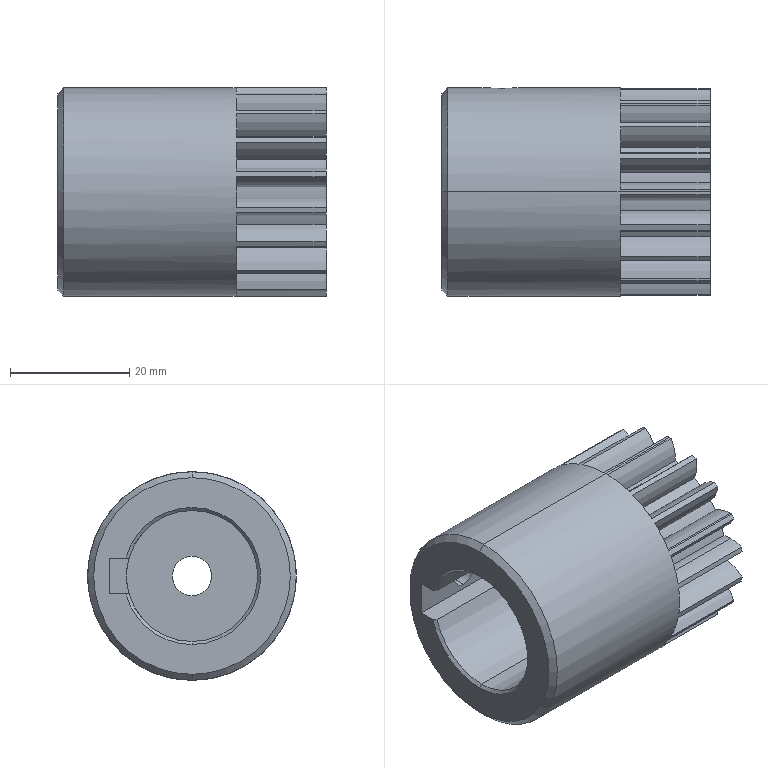Part | SolidWorks | features ICE 3, Chamfer 2, HoleWzd 2, BaseBody 1, MoveFace 1 | 1 solid | 99 faces | box 45 x 35 x 35 mm | volume 27246 mm3 | cylinder 68 | plane 26 | cone 5 | commonest cylinder face diameters 12.6 x40 27.123 x18 4.2 x2 6.6 x2 11 x2 22 x2